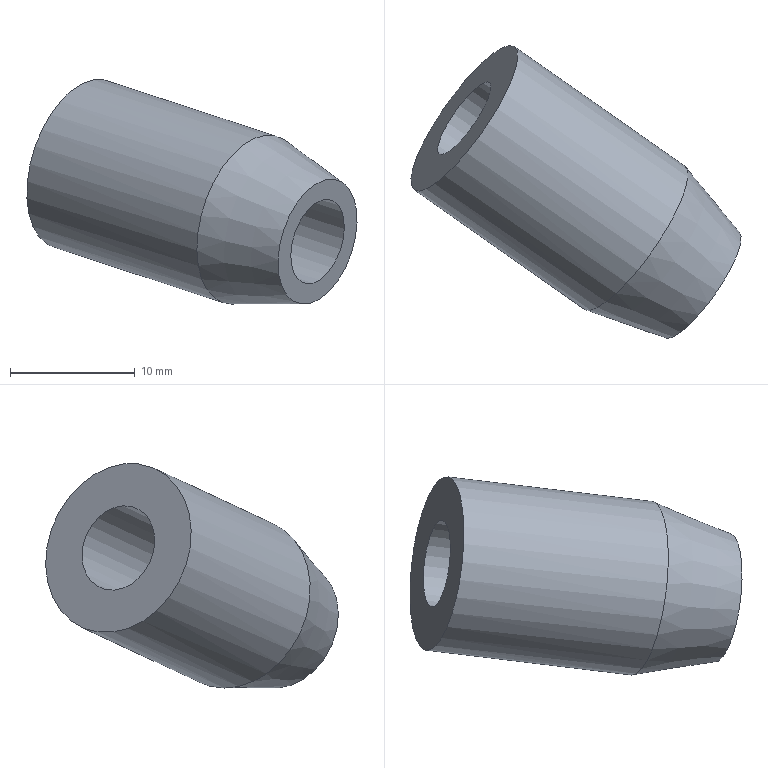Part | NX | features solid 2 | 1 solid | 5 faces | box 26.437 x 23.435 x 17.975 mm | volume 2522 mm3 | plane 2 | cylinder 2 | cone 1 | commonest cylinder face diameters 7 x1 14 x1
STEP:
#1=CARTESIAN_POINT('',(-104.125,729.099,8.856));
#2=VERTEX_POINT('',#1);
#3=CARTESIAN_POINT('',(-108.14,723.365,8.856));
#4=DIRECTION('',(0.7912,-0.554,-0.2588));
#5=DIRECTION('',(0.5736,0.8192,0.));
#6=AXIS2_PLACEMENT_3D('',#3,#4,#5);
#7=CIRCLE('',#6,7.);
#8=EDGE_CURVE('',#2,#2,#7,.T.);
#9=ORIENTED_EDGE('',*,*,#8,.F.);
#10=EDGE_LOOP('',(#9));
#11=FACE_BOUND('',#10,.T.);
#12=CARTESIAN_POINT('',(-110.084,721.705,6.466));
#13=VERTEX_POINT('',#12);
#14=CARTESIAN_POINT('',(-108.14,723.365,8.856));
#15=DIRECTION('',(0.7912,-0.554,-0.2588));
#16=DIRECTION('',(-0.5555,-0.4743,-0.683));
#17=AXIS2_PLACEMENT_3D('',#14,#15,#16);
#18=CIRCLE('',#17,3.5);
#19=EDGE_CURVE('',#13,#13,#18,.T.);
#20=ORIENTED_EDGE('',*,*,#19,.T.);
#21=EDGE_LOOP('',(#20));
#22=FACE_BOUND('',#21,.T.);
#23=CARTESIAN_POINT('',(-108.14,723.365,8.856));
#24=DIRECTION('',(-0.7912,0.554,0.2588));
#25=DIRECTION('',(-0.5555,-0.4743,-0.683));
#26=AXIS2_PLACEMENT_3D('',#23,#24,#25);
#27=PLANE('',#26);
#28=ADVANCED_FACE('',(#11,#22),#27,.T.);
#29=CARTESIAN_POINT('',(-92.027,707.613,-0.8921));
#30=VERTEX_POINT('',#29);
#31=CARTESIAN_POINT('',(-89.15,710.069,2.645));
#32=DIRECTION('',(0.7912,-0.554,-0.2588));
#33=DIRECTION('',(-0.5555,-0.4743,-0.683));
#34=AXIS2_PLACEMENT_3D('',#31,#32,#33);
#35=CIRCLE('',#34,5.178);
#36=EDGE_CURVE('',#30,#30,#35,.F.);
#37=ORIENTED_EDGE('',*,*,#36,.F.);
#38=EDGE_LOOP('',(#37));
#39=FACE_BOUND('',#38,.T.);
#40=CARTESIAN_POINT('',(-91.094,708.409,0.2541));
#41=VERTEX_POINT('',#40);
#42=CARTESIAN_POINT('',(-89.15,710.069,2.645));
#43=DIRECTION('',(0.7912,-0.554,-0.2588));
#44=DIRECTION('',(-0.5555,-0.4743,-0.683));
#45=AXIS2_PLACEMENT_3D('',#42,#43,#44);
#46=CIRCLE('',#45,3.5);
#47=EDGE_CURVE('',#41,#41,#46,.T.);
#48=ORIENTED_EDGE('',*,*,#47,.F.);
#49=EDGE_LOOP('',(#48));
#50=FACE_BOUND('',#49,.T.);
#51=CARTESIAN_POINT('',(-89.15,710.069,2.645));
#52=DIRECTION('',(-0.7912,0.554,0.2588));
#53=DIRECTION('',(-0.5555,-0.4743,-0.683));
#54=AXIS2_PLACEMENT_3D('',#51,#52,#53);
#55=PLANE('',#54);
#56=ADVANCED_FACE('',(#39,#50),#55,.F.);
#57=CARTESIAN_POINT('',(-90.515,719.57,4.404));
#58=VERTEX_POINT('',#57);
#59=CARTESIAN_POINT('',(-94.53,713.835,4.404));
#60=DIRECTION('',(0.7912,-0.554,-0.2588));
#61=DIRECTION('',(0.5736,0.8192,0.));
#62=AXIS2_PLACEMENT_3D('',#59,#60,#61);
#63=CIRCLE('',#62,7.);
#64=EDGE_CURVE('',#58,#58,#63,.T.);
#65=ORIENTED_EDGE('',*,*,#64,.F.);
#66=EDGE_LOOP('',(#65));
#67=FACE_BOUND('',#66,.T.);
#68=ORIENTED_EDGE('',*,*,#8,.T.);
#69=EDGE_LOOP('',(#68));
#70=FACE_BOUND('',#69,.T.);
#71=CARTESIAN_POINT('',(-108.14,723.365,8.856));
#72=DIRECTION('',(0.7912,-0.554,-0.2588));
#73=DIRECTION('',(0.5555,0.4743,0.683));
#74=AXIS2_PLACEMENT_3D('',#71,#72,#73);
#75=CYLINDRICAL_SURFACE('',#74,7.);
#76=ADVANCED_FACE('',(#67,#70),#75,.T.);
#77=ORIENTED_EDGE('',*,*,#19,.F.);
#78=EDGE_LOOP('',(#77));
#79=FACE_BOUND('',#78,.T.);
#80=ORIENTED_EDGE('',*,*,#47,.T.);
#81=EDGE_LOOP('',(#80));
#82=FACE_BOUND('',#81,.T.);
#83=CARTESIAN_POINT('',(-108.14,723.365,8.856));
#84=DIRECTION('',(0.7912,-0.554,-0.2588));
#85=DIRECTION('',(0.5555,0.4743,0.683));
#86=AXIS2_PLACEMENT_3D('',#83,#84,#85);
#87=CYLINDRICAL_SURFACE('',#86,3.5);
#88=ADVANCED_FACE('',(#79,#82),#87,.F.);
#89=ORIENTED_EDGE('',*,*,#36,.T.);
#90=EDGE_LOOP('',(#89));
#91=FACE_BOUND('',#90,.T.);
#92=ORIENTED_EDGE('',*,*,#64,.T.);
#93=EDGE_LOOP('',(#92));
#94=FACE_BOUND('',#93,.T.);
#95=CARTESIAN_POINT('',(-92.315,712.285,3.68));
#96=DIRECTION('',(-0.7912,0.554,0.2588));
#97=DIRECTION('',(-0.5555,-0.4743,-0.683));
#98=AXIS2_PLACEMENT_3D('',#95,#96,#97);
#99=CONICAL_SURFACE('',#98,6.25,0.2618);
#100=ADVANCED_FACE('',(#91,#94),#99,.T.);
#101=CLOSED_SHELL('',(#28,#56,#76,#88,#100));
#102=MANIFOLD_SOLID_BREP('',#101);
#103=(LENGTH_UNIT()NAMED_UNIT(*)SI_UNIT(.MILLI.,.METRE.));
#104=UNCERTAINTY_MEASURE_WITH_UNIT(LENGTH_MEASURE(0.00001),#103,'','');
#105=(NAMED_UNIT(*)PLANE_ANGLE_UNIT()SI_UNIT($,.RADIAN.));
#106=(NAMED_UNIT(*)SI_UNIT($,.STERADIAN.)SOLID_ANGLE_UNIT());
#107=(GEOMETRIC_REPRESENTATION_CONTEXT(3)GLOBAL_UNCERTAINTY_ASSIGNED_CONTEXT((#104))GLOBAL_UNIT_ASSIGNED_CONTEXT((#103,#105,#106))REPRESENTATION_CONTEXT('',''));
#108=ADVANCED_BREP_SHAPE_REPRESENTATION('',(#102),#107);